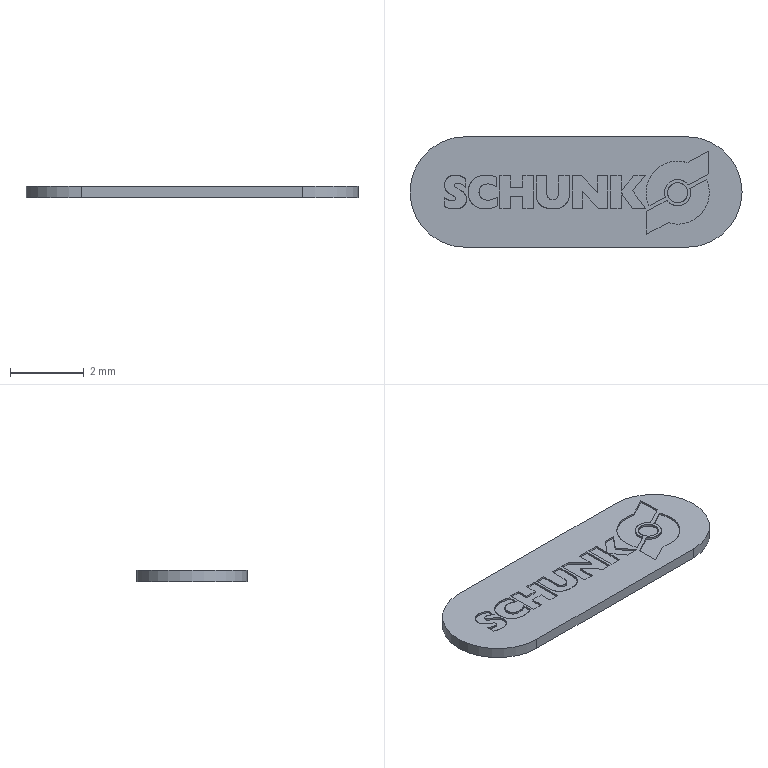Part | SolidWorks | features BaseBody 1 | 1 solid | 815 faces | box 9 x 3 x 0.3 mm | volume 7.24 mm3 | plane 809 | cylinder 6 | commonest cylinder face diameters 3 x3 0.048 x2 0.052 x1